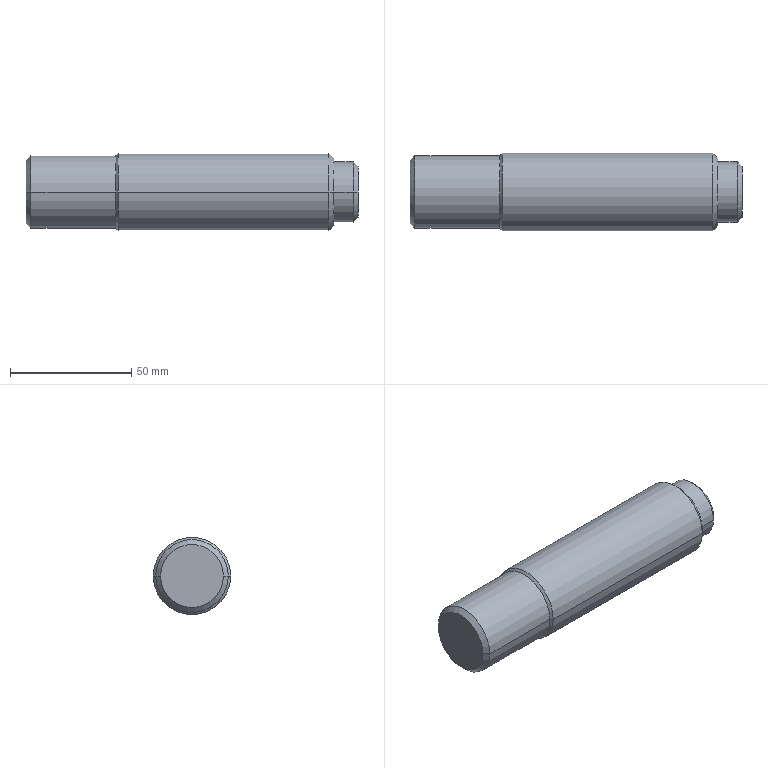Part | SolidWorks | features BaseBody 1 | 1 solid | 17 faces | box 137 x 32 x 32 mm | volume 102874 mm3 | cone 8 | cylinder 6 | plane 3 | commonest cylinder face diameters 25 x2 30 x2 32 x2
STEP:
#1=CARTESIAN_POINT('',(-0.4,16.,0.));
#2=VERTEX_POINT('',#1);
#3=CARTESIAN_POINT('',(-0.4,-16.,0.));
#4=VERTEX_POINT('',#3);
#5=CARTESIAN_POINT('',(-0.4,0.,0.));
#6=DIRECTION('',(1.,0.,0.));
#7=DIRECTION('',(0.,1.,0.));
#8=AXIS2_PLACEMENT_3D('',#5,#6,#7);
#9=CIRCLE('',#8,16.);
#10=EDGE_CURVE('',#2,#4,#9,.T.);
#11=ORIENTED_EDGE('',*,*,#10,.T.);
#12=CARTESIAN_POINT('',(86.6,-16.,0.));
#13=VERTEX_POINT('',#12);
#14=CARTESIAN_POINT('',(44.1,-16.,0.));
#15=DIRECTION('',(1.,0.,0.));
#16=VECTOR('',#15,1000.);
#17=LINE('',#14,#16);
#18=EDGE_CURVE('',#4,#13,#17,.T.);
#19=ORIENTED_EDGE('',*,*,#18,.T.);
#20=CARTESIAN_POINT('',(86.6,16.,0.));
#21=VERTEX_POINT('',#20);
#22=CARTESIAN_POINT('',(86.6,0.,0.));
#23=DIRECTION('',(-1.,0.,0.));
#24=DIRECTION('',(0.,1.,0.));
#25=AXIS2_PLACEMENT_3D('',#22,#23,#24);
#26=CIRCLE('',#25,16.);
#27=EDGE_CURVE('',#13,#21,#26,.T.);
#28=ORIENTED_EDGE('',*,*,#27,.T.);
#29=CARTESIAN_POINT('',(44.1,16.,0.));
#30=DIRECTION('',(1.,0.,0.));
#31=VECTOR('',#30,1000.);
#32=LINE('',#29,#31);
#33=EDGE_CURVE('',#2,#21,#32,.T.);
#34=ORIENTED_EDGE('',*,*,#33,.F.);
#35=EDGE_LOOP('',(#11,#19,#28,#34));
#36=FACE_OUTER_BOUND('',#35,.T.);
#37=CARTESIAN_POINT('',(44.1,0.,0.));
#38=DIRECTION('',(1.,0.,0.));
#39=DIRECTION('',(0.,1.,0.));
#40=AXIS2_PLACEMENT_3D('',#37,#38,#39);
#41=CYLINDRICAL_SURFACE('',#40,16.);
#42=ADVANCED_FACE('',(#36),#41,.T.);
#43=CARTESIAN_POINT('',(88.6,-14.,0.));
#44=VERTEX_POINT('',#43);
#45=CARTESIAN_POINT('',(88.6,14.,0.));
#46=VERTEX_POINT('',#45);
#47=CARTESIAN_POINT('',(88.6,0.,0.));
#48=DIRECTION('',(-1.,0.,0.));
#49=DIRECTION('',(0.,-1.,0.));
#50=AXIS2_PLACEMENT_3D('',#47,#48,#49);
#51=CIRCLE('',#50,14.);
#52=EDGE_CURVE('',#44,#46,#51,.T.);
#53=ORIENTED_EDGE('',*,*,#52,.T.);
#54=CARTESIAN_POINT('',(86.6,16.,0.));
#55=DIRECTION('',(-0.7071,0.7071,0.));
#56=VECTOR('',#55,1000.);
#57=LINE('',#54,#56);
#58=EDGE_CURVE('',#46,#21,#57,.T.);
#59=ORIENTED_EDGE('',*,*,#58,.T.);
#60=ORIENTED_EDGE('',*,*,#27,.F.);
#61=CARTESIAN_POINT('',(86.6,-16.,0.));
#62=DIRECTION('',(-0.7071,-0.7071,0.));
#63=VECTOR('',#62,1000.);
#64=LINE('',#61,#63);
#65=EDGE_CURVE('',#44,#13,#64,.T.);
#66=ORIENTED_EDGE('',*,*,#65,.F.);
#67=EDGE_LOOP('',(#53,#59,#60,#66));
#68=FACE_OUTER_BOUND('',#67,.T.);
#69=CARTESIAN_POINT('',(86.6,0.,0.));
#70=DIRECTION('',(-1.,0.,0.));
#71=DIRECTION('',(0.,-1.,0.));
#72=AXIS2_PLACEMENT_3D('',#69,#70,#71);
#73=CONICAL_SURFACE('',#72,16.,0.7854);
#74=ADVANCED_FACE('',(#68),#73,.T.);
#75=CARTESIAN_POINT('',(-1.4,15.,0.));
#76=VERTEX_POINT('',#75);
#77=CARTESIAN_POINT('',(-1.4,-15.,0.));
#78=VERTEX_POINT('',#77);
#79=CARTESIAN_POINT('',(-1.4,0.,0.));
#80=DIRECTION('',(1.,0.,0.));
#81=DIRECTION('',(0.,1.,0.));
#82=AXIS2_PLACEMENT_3D('',#79,#80,#81);
#83=CIRCLE('',#82,15.);
#84=EDGE_CURVE('',#76,#78,#83,.T.);
#85=ORIENTED_EDGE('',*,*,#84,.T.);
#86=CARTESIAN_POINT('',(-0.4,-16.,0.));
#87=DIRECTION('',(0.7071,-0.7071,0.));
#88=VECTOR('',#87,1000.);
#89=LINE('',#86,#88);
#90=EDGE_CURVE('',#78,#4,#89,.T.);
#91=ORIENTED_EDGE('',*,*,#90,.T.);
#92=ORIENTED_EDGE('',*,*,#10,.F.);
#93=CARTESIAN_POINT('',(-0.4,16.,0.));
#94=DIRECTION('',(0.7071,0.7071,0.));
#95=VECTOR('',#94,1000.);
#96=LINE('',#93,#95);
#97=EDGE_CURVE('',#76,#2,#96,.T.);
#98=ORIENTED_EDGE('',*,*,#97,.F.);
#99=EDGE_LOOP('',(#85,#91,#92,#98));
#100=FACE_OUTER_BOUND('',#99,.T.);
#101=CARTESIAN_POINT('',(-0.4,0.,0.));
#102=DIRECTION('',(1.,0.,0.));
#103=DIRECTION('',(0.,1.,0.));
#104=AXIS2_PLACEMENT_3D('',#101,#102,#103);
#105=CONICAL_SURFACE('',#104,16.,0.7854);
#106=ADVANCED_FACE('',(#100),#105,.T.);
#107=CARTESIAN_POINT('',(-36.4,15.,0.));
#108=VERTEX_POINT('',#107);
#109=CARTESIAN_POINT('',(-36.4,-15.,0.));
#110=VERTEX_POINT('',#109);
#111=CARTESIAN_POINT('',(-36.4,0.,0.));
#112=DIRECTION('',(1.,0.,0.));
#113=DIRECTION('',(0.,1.,0.));
#114=AXIS2_PLACEMENT_3D('',#111,#112,#113);
#115=CIRCLE('',#114,15.);
#116=EDGE_CURVE('',#108,#110,#115,.T.);
#117=ORIENTED_EDGE('',*,*,#116,.T.);
#118=CARTESIAN_POINT('',(-18.9,-15.,0.));
#119=DIRECTION('',(1.,0.,0.));
#120=VECTOR('',#119,1000.);
#121=LINE('',#118,#120);
#122=EDGE_CURVE('',#110,#78,#121,.T.);
#123=ORIENTED_EDGE('',*,*,#122,.T.);
#124=ORIENTED_EDGE('',*,*,#84,.F.);
#125=CARTESIAN_POINT('',(-18.9,15.,0.));
#126=DIRECTION('',(1.,0.,0.));
#127=VECTOR('',#126,1000.);
#128=LINE('',#125,#127);
#129=EDGE_CURVE('',#108,#76,#128,.T.);
#130=ORIENTED_EDGE('',*,*,#129,.F.);
#131=EDGE_LOOP('',(#117,#123,#124,#130));
#132=FACE_OUTER_BOUND('',#131,.T.);
#133=CARTESIAN_POINT('',(-18.9,0.,0.));
#134=DIRECTION('',(1.,0.,0.));
#135=DIRECTION('',(0.,1.,0.));
#136=AXIS2_PLACEMENT_3D('',#133,#134,#135);
#137=CYLINDRICAL_SURFACE('',#136,15.);
#138=ADVANCED_FACE('',(#132),#137,.T.);
#139=CARTESIAN_POINT('',(88.6,-12.5,0.));
#140=VERTEX_POINT('',#139);
#141=CARTESIAN_POINT('',(88.6,12.5,0.));
#142=VERTEX_POINT('',#141);
#143=CARTESIAN_POINT('',(88.6,0.,0.));
#144=DIRECTION('',(-1.,0.,0.));
#145=DIRECTION('',(0.,1.,0.));
#146=AXIS2_PLACEMENT_3D('',#143,#144,#145);
#147=CIRCLE('',#146,12.5);
#148=EDGE_CURVE('',#140,#142,#147,.T.);
#149=ORIENTED_EDGE('',*,*,#148,.F.);
#150=CARTESIAN_POINT('',(96.6,-12.5,0.));
#151=VERTEX_POINT('',#150);
#152=CARTESIAN_POINT('',(93.6,-12.5,0.));
#153=DIRECTION('',(1.,0.,0.));
#154=VECTOR('',#153,1000.);
#155=LINE('',#152,#154);
#156=EDGE_CURVE('',#140,#151,#155,.T.);
#157=ORIENTED_EDGE('',*,*,#156,.T.);
#158=CARTESIAN_POINT('',(96.6,12.5,0.));
#159=VERTEX_POINT('',#158);
#160=CARTESIAN_POINT('',(96.6,0.,0.));
#161=DIRECTION('',(-1.,0.,0.));
#162=DIRECTION('',(0.,1.,0.));
#163=AXIS2_PLACEMENT_3D('',#160,#161,#162);
#164=CIRCLE('',#163,12.5);
#165=EDGE_CURVE('',#151,#159,#164,.T.);
#166=ORIENTED_EDGE('',*,*,#165,.T.);
#167=CARTESIAN_POINT('',(93.6,12.5,0.));
#168=DIRECTION('',(1.,0.,0.));
#169=VECTOR('',#168,1000.);
#170=LINE('',#167,#169);
#171=EDGE_CURVE('',#142,#159,#170,.T.);
#172=ORIENTED_EDGE('',*,*,#171,.F.);
#173=EDGE_LOOP('',(#149,#157,#166,#172));
#174=FACE_OUTER_BOUND('',#173,.T.);
#175=CARTESIAN_POINT('',(93.6,0.,0.));
#176=DIRECTION('',(1.,0.,0.));
#177=DIRECTION('',(0.,1.,0.));
#178=AXIS2_PLACEMENT_3D('',#175,#176,#177);
#179=CYLINDRICAL_SURFACE('',#178,12.5);
#180=ADVANCED_FACE('',(#174),#179,.T.);
#181=CARTESIAN_POINT('',(-38.4,13.,0.));
#182=VERTEX_POINT('',#181);
#183=CARTESIAN_POINT('',(-38.4,-13.,0.));
#184=VERTEX_POINT('',#183);
#185=CARTESIAN_POINT('',(-38.4,0.,0.));
#186=DIRECTION('',(1.,0.,0.));
#187=DIRECTION('',(0.,1.,0.));
#188=AXIS2_PLACEMENT_3D('',#185,#186,#187);
#189=CIRCLE('',#188,13.);
#190=EDGE_CURVE('',#182,#184,#189,.T.);
#191=ORIENTED_EDGE('',*,*,#190,.T.);
#192=CARTESIAN_POINT('',(-36.4,-15.,0.));
#193=DIRECTION('',(0.7071,-0.7071,0.));
#194=VECTOR('',#193,1000.);
#195=LINE('',#192,#194);
#196=EDGE_CURVE('',#184,#110,#195,.T.);
#197=ORIENTED_EDGE('',*,*,#196,.T.);
#198=ORIENTED_EDGE('',*,*,#116,.F.);
#199=CARTESIAN_POINT('',(-36.4,15.,0.));
#200=DIRECTION('',(0.7071,0.7071,0.));
#201=VECTOR('',#200,1000.);
#202=LINE('',#199,#201);
#203=EDGE_CURVE('',#182,#108,#202,.T.);
#204=ORIENTED_EDGE('',*,*,#203,.F.);
#205=EDGE_LOOP('',(#191,#197,#198,#204));
#206=FACE_OUTER_BOUND('',#205,.T.);
#207=CARTESIAN_POINT('',(-36.4,0.,0.));
#208=DIRECTION('',(1.,0.,0.));
#209=DIRECTION('',(0.,1.,0.));
#210=AXIS2_PLACEMENT_3D('',#207,#208,#209);
#211=CONICAL_SURFACE('',#210,15.,0.7854);
#212=ADVANCED_FACE('',(#206),#211,.T.);
#213=CARTESIAN_POINT('',(98.6,-10.5,0.));
#214=VERTEX_POINT('',#213);
#215=CARTESIAN_POINT('',(98.6,10.5,0.));
#216=VERTEX_POINT('',#215);
#217=CARTESIAN_POINT('',(98.6,0.,0.));
#218=DIRECTION('',(-1.,0.,0.));
#219=DIRECTION('',(0.,-1.,0.));
#220=AXIS2_PLACEMENT_3D('',#217,#218,#219);
#221=CIRCLE('',#220,10.5);
#222=EDGE_CURVE('',#214,#216,#221,.T.);
#223=ORIENTED_EDGE('',*,*,#222,.T.);
#224=CARTESIAN_POINT('',(96.6,12.5,0.));
#225=DIRECTION('',(-0.7071,0.7071,0.));
#226=VECTOR('',#225,1000.);
#227=LINE('',#224,#226);
#228=EDGE_CURVE('',#216,#159,#227,.T.);
#229=ORIENTED_EDGE('',*,*,#228,.T.);
#230=ORIENTED_EDGE('',*,*,#165,.F.);
#231=CARTESIAN_POINT('',(96.6,-12.5,0.));
#232=DIRECTION('',(-0.7071,-0.7071,0.));
#233=VECTOR('',#232,1000.);
#234=LINE('',#231,#233);
#235=EDGE_CURVE('',#214,#151,#234,.T.);
#236=ORIENTED_EDGE('',*,*,#235,.F.);
#237=EDGE_LOOP('',(#223,#229,#230,#236));
#238=FACE_OUTER_BOUND('',#237,.T.);
#239=CARTESIAN_POINT('',(96.6,0.,0.));
#240=DIRECTION('',(-1.,0.,0.));
#241=DIRECTION('',(0.,-1.,0.));
#242=AXIS2_PLACEMENT_3D('',#239,#240,#241);
#243=CONICAL_SURFACE('',#242,12.5,0.7854);
#244=ADVANCED_FACE('',(#238),#243,.T.);
#245=ORIENTED_EDGE('',*,*,#18,.F.);
#246=CARTESIAN_POINT('',(-0.4,0.,0.));
#247=DIRECTION('',(1.,0.,0.));
#248=DIRECTION('',(0.,1.,0.));
#249=AXIS2_PLACEMENT_3D('',#246,#247,#248);
#250=CIRCLE('',#249,16.);
#251=EDGE_CURVE('',#4,#2,#250,.T.);
#252=ORIENTED_EDGE('',*,*,#251,.T.);
#253=ORIENTED_EDGE('',*,*,#33,.T.);
#254=CARTESIAN_POINT('',(86.6,0.,0.));
#255=DIRECTION('',(-1.,0.,0.));
#256=DIRECTION('',(0.,1.,0.));
#257=AXIS2_PLACEMENT_3D('',#254,#255,#256);
#258=CIRCLE('',#257,16.);
#259=EDGE_CURVE('',#21,#13,#258,.T.);
#260=ORIENTED_EDGE('',*,*,#259,.T.);
#261=EDGE_LOOP('',(#245,#252,#253,#260));
#262=FACE_OUTER_BOUND('',#261,.T.);
#263=CARTESIAN_POINT('',(44.1,0.,0.));
#264=DIRECTION('',(1.,0.,0.));
#265=DIRECTION('',(0.,1.,0.));
#266=AXIS2_PLACEMENT_3D('',#263,#264,#265);
#267=CYLINDRICAL_SURFACE('',#266,16.);
#268=ADVANCED_FACE('',(#262),#267,.T.);
#269=ORIENTED_EDGE('',*,*,#58,.F.);
#270=CARTESIAN_POINT('',(88.6,0.,0.));
#271=DIRECTION('',(-1.,0.,0.));
#272=DIRECTION('',(0.,-1.,0.));
#273=AXIS2_PLACEMENT_3D('',#270,#271,#272);
#274=CIRCLE('',#273,14.);
#275=EDGE_CURVE('',#46,#44,#274,.T.);
#276=ORIENTED_EDGE('',*,*,#275,.T.);
#277=ORIENTED_EDGE('',*,*,#65,.T.);
#278=ORIENTED_EDGE('',*,*,#259,.F.);
#279=EDGE_LOOP('',(#269,#276,#277,#278));
#280=FACE_OUTER_BOUND('',#279,.T.);
#281=CARTESIAN_POINT('',(86.6,0.,0.));
#282=DIRECTION('',(-1.,0.,0.));
#283=DIRECTION('',(0.,-1.,0.));
#284=AXIS2_PLACEMENT_3D('',#281,#282,#283);
#285=CONICAL_SURFACE('',#284,16.,0.7854);
#286=ADVANCED_FACE('',(#280),#285,.T.);
#287=ORIENTED_EDGE('',*,*,#90,.F.);
#288=CARTESIAN_POINT('',(-1.4,0.,0.));
#289=DIRECTION('',(1.,0.,0.));
#290=DIRECTION('',(0.,1.,0.));
#291=AXIS2_PLACEMENT_3D('',#288,#289,#290);
#292=CIRCLE('',#291,15.);
#293=EDGE_CURVE('',#78,#76,#292,.T.);
#294=ORIENTED_EDGE('',*,*,#293,.T.);
#295=ORIENTED_EDGE('',*,*,#97,.T.);
#296=ORIENTED_EDGE('',*,*,#251,.F.);
#297=EDGE_LOOP('',(#287,#294,#295,#296));
#298=FACE_OUTER_BOUND('',#297,.T.);
#299=CARTESIAN_POINT('',(-0.4,0.,0.));
#300=DIRECTION('',(1.,0.,0.));
#301=DIRECTION('',(0.,1.,0.));
#302=AXIS2_PLACEMENT_3D('',#299,#300,#301);
#303=CONICAL_SURFACE('',#302,16.,0.7854);
#304=ADVANCED_FACE('',(#298),#303,.T.);
#305=CARTESIAN_POINT('',(88.6,0.,0.));
#306=DIRECTION('',(-1.,0.,0.));
#307=DIRECTION('',(0.,1.,0.));
#308=AXIS2_PLACEMENT_3D('',#305,#306,#307);
#309=CIRCLE('',#308,12.5);
#310=EDGE_CURVE('',#142,#140,#309,.T.);
#311=ORIENTED_EDGE('',*,*,#310,.T.);
#312=ORIENTED_EDGE('',*,*,#148,.T.);
#313=EDGE_LOOP('',(#311,#312));
#314=FACE_BOUND('',#313,.T.);
#315=ORIENTED_EDGE('',*,*,#52,.F.);
#316=ORIENTED_EDGE('',*,*,#275,.F.);
#317=EDGE_LOOP('',(#315,#316));
#318=FACE_OUTER_BOUND('',#317,.T.);
#319=CARTESIAN_POINT('',(88.6,12.5,0.));
#320=DIRECTION('',(1.,0.,0.));
#321=DIRECTION('',(0.,1.,0.));
#322=AXIS2_PLACEMENT_3D('',#319,#320,#321);
#323=PLANE('',#322);
#324=ADVANCED_FACE('',(#314,#318),#323,.T.);
#325=ORIENTED_EDGE('',*,*,#122,.F.);
#326=CARTESIAN_POINT('',(-36.4,0.,0.));
#327=DIRECTION('',(1.,0.,0.));
#328=DIRECTION('',(0.,1.,0.));
#329=AXIS2_PLACEMENT_3D('',#326,#327,#328);
#330=CIRCLE('',#329,15.);
#331=EDGE_CURVE('',#110,#108,#330,.T.);
#332=ORIENTED_EDGE('',*,*,#331,.T.);
#333=ORIENTED_EDGE('',*,*,#129,.T.);
#334=ORIENTED_EDGE('',*,*,#293,.F.);
#335=EDGE_LOOP('',(#325,#332,#333,#334));
#336=FACE_OUTER_BOUND('',#335,.T.);
#337=CARTESIAN_POINT('',(-18.9,0.,0.));
#338=DIRECTION('',(1.,0.,0.));
#339=DIRECTION('',(0.,1.,0.));
#340=AXIS2_PLACEMENT_3D('',#337,#338,#339);
#341=CYLINDRICAL_SURFACE('',#340,15.);
#342=ADVANCED_FACE('',(#336),#341,.T.);
#343=ORIENTED_EDGE('',*,*,#156,.F.);
#344=ORIENTED_EDGE('',*,*,#310,.F.);
#345=ORIENTED_EDGE('',*,*,#171,.T.);
#346=CARTESIAN_POINT('',(96.6,0.,0.));
#347=DIRECTION('',(-1.,0.,0.));
#348=DIRECTION('',(0.,1.,0.));
#349=AXIS2_PLACEMENT_3D('',#346,#347,#348);
#350=CIRCLE('',#349,12.5);
#351=EDGE_CURVE('',#159,#151,#350,.T.);
#352=ORIENTED_EDGE('',*,*,#351,.T.);
#353=EDGE_LOOP('',(#343,#344,#345,#352));
#354=FACE_OUTER_BOUND('',#353,.T.);
#355=CARTESIAN_POINT('',(93.6,0.,0.));
#356=DIRECTION('',(1.,0.,0.));
#357=DIRECTION('',(0.,1.,0.));
#358=AXIS2_PLACEMENT_3D('',#355,#356,#357);
#359=CYLINDRICAL_SURFACE('',#358,12.5);
#360=ADVANCED_FACE('',(#354),#359,.T.);
#361=ORIENTED_EDGE('',*,*,#196,.F.);
#362=CARTESIAN_POINT('',(-38.4,0.,0.));
#363=DIRECTION('',(1.,0.,0.));
#364=DIRECTION('',(0.,1.,0.));
#365=AXIS2_PLACEMENT_3D('',#362,#363,#364);
#366=CIRCLE('',#365,13.);
#367=EDGE_CURVE('',#184,#182,#366,.T.);
#368=ORIENTED_EDGE('',*,*,#367,.T.);
#369=ORIENTED_EDGE('',*,*,#203,.T.);
#370=ORIENTED_EDGE('',*,*,#331,.F.);
#371=EDGE_LOOP('',(#361,#368,#369,#370));
#372=FACE_OUTER_BOUND('',#371,.T.);
#373=CARTESIAN_POINT('',(-36.4,0.,0.));
#374=DIRECTION('',(1.,0.,0.));
#375=DIRECTION('',(0.,1.,0.));
#376=AXIS2_PLACEMENT_3D('',#373,#374,#375);
#377=CONICAL_SURFACE('',#376,15.,0.7854);
#378=ADVANCED_FACE('',(#372),#377,.T.);
#379=ORIENTED_EDGE('',*,*,#228,.F.);
#380=CARTESIAN_POINT('',(98.6,0.,0.));
#381=DIRECTION('',(-1.,0.,0.));
#382=DIRECTION('',(0.,-1.,0.));
#383=AXIS2_PLACEMENT_3D('',#380,#381,#382);
#384=CIRCLE('',#383,10.5);
#385=EDGE_CURVE('',#216,#214,#384,.T.);
#386=ORIENTED_EDGE('',*,*,#385,.T.);
#387=ORIENTED_EDGE('',*,*,#235,.T.);
#388=ORIENTED_EDGE('',*,*,#351,.F.);
#389=EDGE_LOOP('',(#379,#386,#387,#388));
#390=FACE_OUTER_BOUND('',#389,.T.);
#391=CARTESIAN_POINT('',(96.6,0.,0.));
#392=DIRECTION('',(-1.,0.,0.));
#393=DIRECTION('',(0.,-1.,0.));
#394=AXIS2_PLACEMENT_3D('',#391,#392,#393);
#395=CONICAL_SURFACE('',#394,12.5,0.7854);
#396=ADVANCED_FACE('',(#390),#395,.T.);
#397=ORIENTED_EDGE('',*,*,#190,.F.);
#398=ORIENTED_EDGE('',*,*,#367,.F.);
#399=EDGE_LOOP('',(#397,#398));
#400=FACE_OUTER_BOUND('',#399,.T.);
#401=CARTESIAN_POINT('',(-38.4,13.,0.));
#402=DIRECTION('',(-1.,0.,0.));
#403=DIRECTION('',(0.,-1.,0.));
#404=AXIS2_PLACEMENT_3D('',#401,#402,#403);
#405=PLANE('',#404);
#406=ADVANCED_FACE('',(#400),#405,.T.);
#407=ORIENTED_EDGE('',*,*,#222,.F.);
#408=ORIENTED_EDGE('',*,*,#385,.F.);
#409=EDGE_LOOP('',(#407,#408));
#410=FACE_OUTER_BOUND('',#409,.T.);
#411=CARTESIAN_POINT('',(98.6,0.,0.));
#412=DIRECTION('',(1.,0.,0.));
#413=DIRECTION('',(0.,1.,0.));
#414=AXIS2_PLACEMENT_3D('',#411,#412,#413);
#415=PLANE('',#414);
#416=ADVANCED_FACE('',(#410),#415,.T.);
#417=CLOSED_SHELL('',(#42,#74,#106,#138,#180,#212,#244,#268,#286,#304,#324,#342,#360,#378,#396,#406,#416));
#418=MANIFOLD_SOLID_BREP('',#417);
#419=CARTESIAN_POINT('',(0.,0.,0.));
#420=DIRECTION('',(0.,0.,1.));
#421=DIRECTION('',(1.,0.,0.));
#422=AXIS2_PLACEMENT_3D('',#419,#420,#421);
#423=(LENGTH_UNIT()NAMED_UNIT(*)SI_UNIT(.MILLI.,.METRE.));
#424=UNCERTAINTY_MEASURE_WITH_UNIT(LENGTH_MEASURE(0.00001),#423,'','');
#425=(NAMED_UNIT(*)PLANE_ANGLE_UNIT()SI_UNIT($,.RADIAN.));
#426=(NAMED_UNIT(*)SI_UNIT($,.STERADIAN.)SOLID_ANGLE_UNIT());
#427=(GEOMETRIC_REPRESENTATION_CONTEXT(3)GLOBAL_UNCERTAINTY_ASSIGNED_CONTEXT((#424))GLOBAL_UNIT_ASSIGNED_CONTEXT((#423,#425,#426))REPRESENTATION_CONTEXT('',''));
#428=ADVANCED_BREP_SHAPE_REPRESENTATION('',(#418,#422),#427);